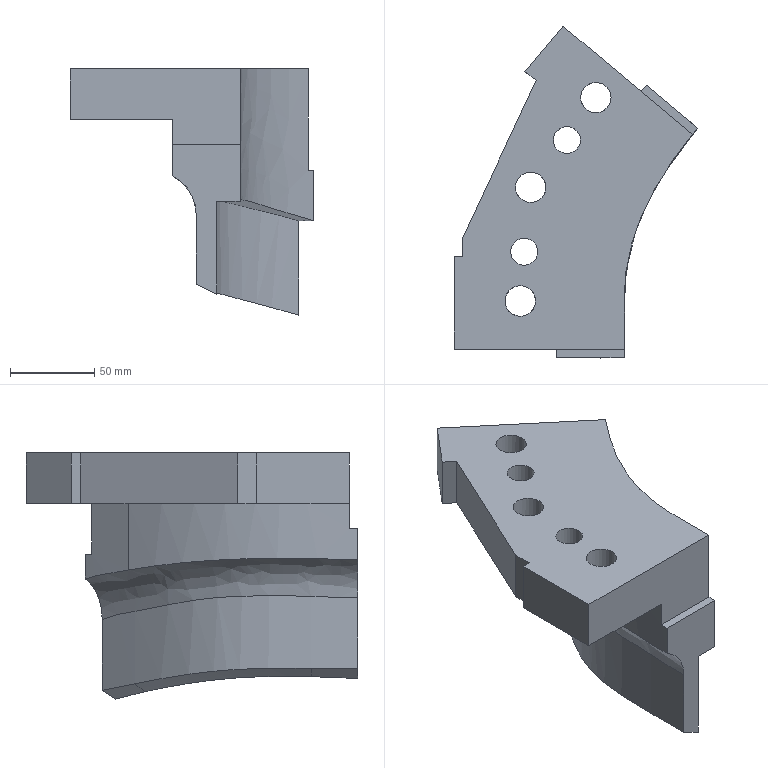Part | NX | features solid 2 | 1 solid | 35 faces | box 143.978 x 196.403 x 145.873 mm | volume 836095 mm3 | plane 17 | spline 10 | cylinder 8 | commonest cylinder face diameters 18 x3 26 x3 16 x2